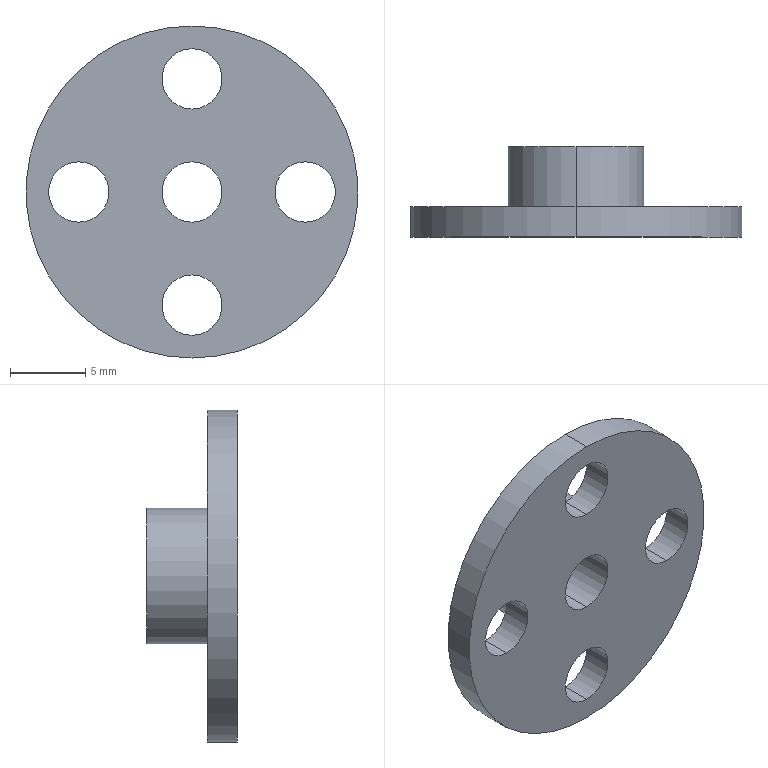Part | SolidWorks | features ICE 2, Extrusion 1 | 1 solid | 17 faces | box 22 x 6 x 22 mm | volume 838.805 mm3 | cylinder 14 | plane 3 | commonest cylinder face diameters 4 x10 9 x2 22 x2
STEP:
#1=CARTESIAN_POINT('',(0.,0.,-2.));
#2=VERTEX_POINT('',#1);
#3=CARTESIAN_POINT('',(0.,0.,2.));
#4=VERTEX_POINT('',#3);
#5=CARTESIAN_POINT('',(0.,0.,0.));
#6=DIRECTION('',(0.,1.,0.));
#7=DIRECTION('',(0.,0.,1.));
#8=AXIS2_PLACEMENT_3D('',#5,#6,#7);
#9=CIRCLE('',#8,2.);
#10=EDGE_CURVE('',#2,#4,#9,.T.);
#11=ORIENTED_EDGE('',*,*,#10,.F.);
#12=CARTESIAN_POINT('',(0.,6.,-2.));
#13=VERTEX_POINT('',#12);
#14=CARTESIAN_POINT('',(0.,0.,-2.));
#15=DIRECTION('',(0.,1.,0.));
#16=VECTOR('',#15,1000.);
#17=LINE('',#14,#16);
#18=EDGE_CURVE('',#2,#13,#17,.T.);
#19=ORIENTED_EDGE('',*,*,#18,.T.);
#20=CARTESIAN_POINT('',(0.,6.,2.));
#21=VERTEX_POINT('',#20);
#22=CARTESIAN_POINT('',(0.,6.,0.));
#23=DIRECTION('',(0.,1.,0.));
#24=DIRECTION('',(0.,0.,1.));
#25=AXIS2_PLACEMENT_3D('',#22,#23,#24);
#26=CIRCLE('',#25,2.);
#27=EDGE_CURVE('',#13,#21,#26,.T.);
#28=ORIENTED_EDGE('',*,*,#27,.T.);
#29=CARTESIAN_POINT('',(0.,0.,2.));
#30=DIRECTION('',(0.,1.,0.));
#31=VECTOR('',#30,1000.);
#32=LINE('',#29,#31);
#33=EDGE_CURVE('',#4,#21,#32,.T.);
#34=ORIENTED_EDGE('',*,*,#33,.F.);
#35=EDGE_LOOP('',(#11,#19,#28,#34));
#36=FACE_OUTER_BOUND('',#35,.T.);
#37=CARTESIAN_POINT('',(0.,0.,0.));
#38=DIRECTION('',(0.,1.,0.));
#39=DIRECTION('',(0.,0.,1.));
#40=AXIS2_PLACEMENT_3D('',#37,#38,#39);
#41=CYLINDRICAL_SURFACE('',#40,2.);
#42=ADVANCED_FACE('',(#36),#41,.F.);
#43=CARTESIAN_POINT('',(0.,6.,4.5));
#44=VERTEX_POINT('',#43);
#45=CARTESIAN_POINT('',(0.,6.,-4.5));
#46=VERTEX_POINT('',#45);
#47=CARTESIAN_POINT('',(0.,6.,0.));
#48=DIRECTION('',(0.,1.,0.));
#49=DIRECTION('',(0.,0.,1.));
#50=AXIS2_PLACEMENT_3D('',#47,#48,#49);
#51=CIRCLE('',#50,4.5);
#52=EDGE_CURVE('',#44,#46,#51,.T.);
#53=ORIENTED_EDGE('',*,*,#52,.F.);
#54=CARTESIAN_POINT('',(0.,2.,4.5));
#55=VERTEX_POINT('',#54);
#56=CARTESIAN_POINT('',(0.,6.,4.5));
#57=DIRECTION('',(0.,-1.,0.));
#58=VECTOR('',#57,1000.);
#59=LINE('',#56,#58);
#60=EDGE_CURVE('',#44,#55,#59,.T.);
#61=ORIENTED_EDGE('',*,*,#60,.T.);
#62=CARTESIAN_POINT('',(0.,2.,-4.5));
#63=VERTEX_POINT('',#62);
#64=CARTESIAN_POINT('',(0.,2.,0.));
#65=DIRECTION('',(0.,1.,0.));
#66=DIRECTION('',(0.,0.,1.));
#67=AXIS2_PLACEMENT_3D('',#64,#65,#66);
#68=CIRCLE('',#67,4.5);
#69=EDGE_CURVE('',#55,#63,#68,.T.);
#70=ORIENTED_EDGE('',*,*,#69,.T.);
#71=CARTESIAN_POINT('',(0.,6.,-4.5));
#72=DIRECTION('',(0.,-1.,0.));
#73=VECTOR('',#72,1000.);
#74=LINE('',#71,#73);
#75=EDGE_CURVE('',#46,#63,#74,.T.);
#76=ORIENTED_EDGE('',*,*,#75,.F.);
#77=EDGE_LOOP('',(#53,#61,#70,#76));
#78=FACE_OUTER_BOUND('',#77,.T.);
#79=CARTESIAN_POINT('',(0.,6.,0.));
#80=DIRECTION('',(0.,-1.,0.));
#81=DIRECTION('',(0.,0.,-1.));
#82=AXIS2_PLACEMENT_3D('',#79,#80,#81);
#83=CYLINDRICAL_SURFACE('',#82,4.5);
#84=ADVANCED_FACE('',(#78),#83,.T.);
#85=CARTESIAN_POINT('',(-7.5,2.,-2.));
#86=VERTEX_POINT('',#85);
#87=CARTESIAN_POINT('',(-7.5,2.,2.));
#88=VERTEX_POINT('',#87);
#89=CARTESIAN_POINT('',(-7.5,2.,0.));
#90=DIRECTION('',(0.,1.,0.));
#91=DIRECTION('',(0.,0.,1.));
#92=AXIS2_PLACEMENT_3D('',#89,#90,#91);
#93=CIRCLE('',#92,2.);
#94=EDGE_CURVE('',#86,#88,#93,.T.);
#95=ORIENTED_EDGE('',*,*,#94,.T.);
#96=CARTESIAN_POINT('',(-7.5,0.,2.));
#97=VERTEX_POINT('',#96);
#98=CARTESIAN_POINT('',(-7.5,2.,2.));
#99=DIRECTION('',(0.,-1.,0.));
#100=VECTOR('',#99,1000.);
#101=LINE('',#98,#100);
#102=EDGE_CURVE('',#88,#97,#101,.T.);
#103=ORIENTED_EDGE('',*,*,#102,.T.);
#104=CARTESIAN_POINT('',(-7.5,0.,-2.));
#105=VERTEX_POINT('',#104);
#106=CARTESIAN_POINT('',(-7.5,0.,0.));
#107=DIRECTION('',(0.,1.,0.));
#108=DIRECTION('',(0.,0.,1.));
#109=AXIS2_PLACEMENT_3D('',#106,#107,#108);
#110=CIRCLE('',#109,2.);
#111=EDGE_CURVE('',#105,#97,#110,.T.);
#112=ORIENTED_EDGE('',*,*,#111,.F.);
#113=CARTESIAN_POINT('',(-7.5,2.,-2.));
#114=DIRECTION('',(0.,-1.,0.));
#115=VECTOR('',#114,1000.);
#116=LINE('',#113,#115);
#117=EDGE_CURVE('',#86,#105,#116,.T.);
#118=ORIENTED_EDGE('',*,*,#117,.F.);
#119=EDGE_LOOP('',(#95,#103,#112,#118));
#120=FACE_OUTER_BOUND('',#119,.T.);
#121=CARTESIAN_POINT('',(-7.5,2.,0.));
#122=DIRECTION('',(0.,-1.,0.));
#123=DIRECTION('',(0.,0.,-1.));
#124=AXIS2_PLACEMENT_3D('',#121,#122,#123);
#125=CYLINDRICAL_SURFACE('',#124,2.);
#126=ADVANCED_FACE('',(#120),#125,.F.);
#127=CARTESIAN_POINT('',(0.,2.,5.5));
#128=VERTEX_POINT('',#127);
#129=CARTESIAN_POINT('',(0.,2.,9.5));
#130=VERTEX_POINT('',#129);
#131=CARTESIAN_POINT('',(0.,2.,7.5));
#132=DIRECTION('',(0.,1.,0.));
#133=DIRECTION('',(0.,0.,1.));
#134=AXIS2_PLACEMENT_3D('',#131,#132,#133);
#135=CIRCLE('',#134,2.);
#136=EDGE_CURVE('',#128,#130,#135,.T.);
#137=ORIENTED_EDGE('',*,*,#136,.T.);
#138=CARTESIAN_POINT('',(0.,0.,9.5));
#139=VERTEX_POINT('',#138);
#140=CARTESIAN_POINT('',(0.,2.,9.5));
#141=DIRECTION('',(0.,-1.,0.));
#142=VECTOR('',#141,1000.);
#143=LINE('',#140,#142);
#144=EDGE_CURVE('',#130,#139,#143,.T.);
#145=ORIENTED_EDGE('',*,*,#144,.T.);
#146=CARTESIAN_POINT('',(0.,0.,5.5));
#147=VERTEX_POINT('',#146);
#148=CARTESIAN_POINT('',(0.,0.,7.5));
#149=DIRECTION('',(0.,1.,0.));
#150=DIRECTION('',(0.,0.,1.));
#151=AXIS2_PLACEMENT_3D('',#148,#149,#150);
#152=CIRCLE('',#151,2.);
#153=EDGE_CURVE('',#147,#139,#152,.T.);
#154=ORIENTED_EDGE('',*,*,#153,.F.);
#155=CARTESIAN_POINT('',(0.,2.,5.5));
#156=DIRECTION('',(0.,-1.,0.));
#157=VECTOR('',#156,1000.);
#158=LINE('',#155,#157);
#159=EDGE_CURVE('',#128,#147,#158,.T.);
#160=ORIENTED_EDGE('',*,*,#159,.F.);
#161=EDGE_LOOP('',(#137,#145,#154,#160));
#162=FACE_OUTER_BOUND('',#161,.T.);
#163=CARTESIAN_POINT('',(0.,2.,7.5));
#164=DIRECTION('',(0.,-1.,0.));
#165=DIRECTION('',(0.,0.,-1.));
#166=AXIS2_PLACEMENT_3D('',#163,#164,#165);
#167=CYLINDRICAL_SURFACE('',#166,2.);
#168=ADVANCED_FACE('',(#162),#167,.F.);
#169=CARTESIAN_POINT('',(7.5,2.,-2.));
#170=VERTEX_POINT('',#169);
#171=CARTESIAN_POINT('',(7.5,2.,2.));
#172=VERTEX_POINT('',#171);
#173=CARTESIAN_POINT('',(7.5,2.,0.));
#174=DIRECTION('',(0.,1.,0.));
#175=DIRECTION('',(0.,0.,1.));
#176=AXIS2_PLACEMENT_3D('',#173,#174,#175);
#177=CIRCLE('',#176,2.);
#178=EDGE_CURVE('',#170,#172,#177,.T.);
#179=ORIENTED_EDGE('',*,*,#178,.T.);
#180=CARTESIAN_POINT('',(7.5,0.,2.));
#181=VERTEX_POINT('',#180);
#182=CARTESIAN_POINT('',(7.5,2.,2.));
#183=DIRECTION('',(0.,-1.,0.));
#184=VECTOR('',#183,1000.);
#185=LINE('',#182,#184);
#186=EDGE_CURVE('',#172,#181,#185,.T.);
#187=ORIENTED_EDGE('',*,*,#186,.T.);
#188=CARTESIAN_POINT('',(7.5,0.,-2.));
#189=VERTEX_POINT('',#188);
#190=CARTESIAN_POINT('',(7.5,0.,0.));
#191=DIRECTION('',(0.,1.,0.));
#192=DIRECTION('',(0.,0.,1.));
#193=AXIS2_PLACEMENT_3D('',#190,#191,#192);
#194=CIRCLE('',#193,2.);
#195=EDGE_CURVE('',#189,#181,#194,.T.);
#196=ORIENTED_EDGE('',*,*,#195,.F.);
#197=CARTESIAN_POINT('',(7.5,2.,-2.));
#198=DIRECTION('',(0.,-1.,0.));
#199=VECTOR('',#198,1000.);
#200=LINE('',#197,#199);
#201=EDGE_CURVE('',#170,#189,#200,.T.);
#202=ORIENTED_EDGE('',*,*,#201,.F.);
#203=EDGE_LOOP('',(#179,#187,#196,#202));
#204=FACE_OUTER_BOUND('',#203,.T.);
#205=CARTESIAN_POINT('',(7.5,2.,0.));
#206=DIRECTION('',(0.,-1.,0.));
#207=DIRECTION('',(0.,0.,-1.));
#208=AXIS2_PLACEMENT_3D('',#205,#206,#207);
#209=CYLINDRICAL_SURFACE('',#208,2.);
#210=ADVANCED_FACE('',(#204),#209,.F.);
#211=CARTESIAN_POINT('',(0.,2.,-9.5));
#212=VERTEX_POINT('',#211);
#213=CARTESIAN_POINT('',(0.,2.,-5.5));
#214=VERTEX_POINT('',#213);
#215=CARTESIAN_POINT('',(0.,2.,-7.5));
#216=DIRECTION('',(0.,1.,0.));
#217=DIRECTION('',(0.,0.,1.));
#218=AXIS2_PLACEMENT_3D('',#215,#216,#217);
#219=CIRCLE('',#218,2.);
#220=EDGE_CURVE('',#212,#214,#219,.T.);
#221=ORIENTED_EDGE('',*,*,#220,.T.);
#222=CARTESIAN_POINT('',(0.,0.,-5.5));
#223=VERTEX_POINT('',#222);
#224=CARTESIAN_POINT('',(0.,2.,-5.5));
#225=DIRECTION('',(0.,-1.,0.));
#226=VECTOR('',#225,1000.);
#227=LINE('',#224,#226);
#228=EDGE_CURVE('',#214,#223,#227,.T.);
#229=ORIENTED_EDGE('',*,*,#228,.T.);
#230=CARTESIAN_POINT('',(0.,0.,-9.5));
#231=VERTEX_POINT('',#230);
#232=CARTESIAN_POINT('',(0.,0.,-7.5));
#233=DIRECTION('',(0.,1.,0.));
#234=DIRECTION('',(0.,0.,1.));
#235=AXIS2_PLACEMENT_3D('',#232,#233,#234);
#236=CIRCLE('',#235,2.);
#237=EDGE_CURVE('',#231,#223,#236,.T.);
#238=ORIENTED_EDGE('',*,*,#237,.F.);
#239=CARTESIAN_POINT('',(0.,2.,-9.5));
#240=DIRECTION('',(0.,-1.,0.));
#241=VECTOR('',#240,1000.);
#242=LINE('',#239,#241);
#243=EDGE_CURVE('',#212,#231,#242,.T.);
#244=ORIENTED_EDGE('',*,*,#243,.F.);
#245=EDGE_LOOP('',(#221,#229,#238,#244));
#246=FACE_OUTER_BOUND('',#245,.T.);
#247=CARTESIAN_POINT('',(0.,2.,-7.5));
#248=DIRECTION('',(0.,-1.,0.));
#249=DIRECTION('',(0.,0.,-1.));
#250=AXIS2_PLACEMENT_3D('',#247,#248,#249);
#251=CYLINDRICAL_SURFACE('',#250,2.);
#252=ADVANCED_FACE('',(#246),#251,.F.);
#253=CARTESIAN_POINT('',(0.,2.,11.));
#254=VERTEX_POINT('',#253);
#255=CARTESIAN_POINT('',(0.,2.,-11.));
#256=VERTEX_POINT('',#255);
#257=CARTESIAN_POINT('',(0.,2.,0.));
#258=DIRECTION('',(0.,1.,0.));
#259=DIRECTION('',(0.,0.,1.));
#260=AXIS2_PLACEMENT_3D('',#257,#258,#259);
#261=CIRCLE('',#260,11.);
#262=EDGE_CURVE('',#254,#256,#261,.T.);
#263=ORIENTED_EDGE('',*,*,#262,.F.);
#264=CARTESIAN_POINT('',(0.,0.,11.));
#265=VERTEX_POINT('',#264);
#266=CARTESIAN_POINT('',(0.,2.,11.));
#267=DIRECTION('',(0.,-1.,0.));
#268=VECTOR('',#267,1000.);
#269=LINE('',#266,#268);
#270=EDGE_CURVE('',#254,#265,#269,.T.);
#271=ORIENTED_EDGE('',*,*,#270,.T.);
#272=CARTESIAN_POINT('',(0.,0.,-11.));
#273=VERTEX_POINT('',#272);
#274=CARTESIAN_POINT('',(0.,0.,0.));
#275=DIRECTION('',(0.,1.,0.));
#276=DIRECTION('',(0.,0.,1.));
#277=AXIS2_PLACEMENT_3D('',#274,#275,#276);
#278=CIRCLE('',#277,11.);
#279=EDGE_CURVE('',#265,#273,#278,.T.);
#280=ORIENTED_EDGE('',*,*,#279,.T.);
#281=CARTESIAN_POINT('',(0.,2.,-11.));
#282=DIRECTION('',(0.,-1.,0.));
#283=VECTOR('',#282,1000.);
#284=LINE('',#281,#283);
#285=EDGE_CURVE('',#256,#273,#284,.T.);
#286=ORIENTED_EDGE('',*,*,#285,.F.);
#287=EDGE_LOOP('',(#263,#271,#280,#286));
#288=FACE_OUTER_BOUND('',#287,.T.);
#289=CARTESIAN_POINT('',(0.,2.,0.));
#290=DIRECTION('',(0.,-1.,0.));
#291=DIRECTION('',(0.,0.,-1.));
#292=AXIS2_PLACEMENT_3D('',#289,#290,#291);
#293=CYLINDRICAL_SURFACE('',#292,11.);
#294=ADVANCED_FACE('',(#288),#293,.T.);
#295=CARTESIAN_POINT('',(0.,2.,0.));
#296=DIRECTION('',(0.,1.,0.));
#297=DIRECTION('',(0.,0.,1.));
#298=AXIS2_PLACEMENT_3D('',#295,#296,#297);
#299=CIRCLE('',#298,4.5);
#300=EDGE_CURVE('',#63,#55,#299,.T.);
#301=ORIENTED_EDGE('',*,*,#300,.F.);
#302=ORIENTED_EDGE('',*,*,#69,.F.);
#303=EDGE_LOOP('',(#301,#302));
#304=FACE_BOUND('',#303,.T.);
#305=ORIENTED_EDGE('',*,*,#136,.F.);
#306=CARTESIAN_POINT('',(0.,2.,7.5));
#307=DIRECTION('',(0.,1.,0.));
#308=DIRECTION('',(0.,0.,1.));
#309=AXIS2_PLACEMENT_3D('',#306,#307,#308);
#310=CIRCLE('',#309,2.);
#311=EDGE_CURVE('',#130,#128,#310,.T.);
#312=ORIENTED_EDGE('',*,*,#311,.F.);
#313=EDGE_LOOP('',(#305,#312));
#314=FACE_BOUND('',#313,.T.);
#315=ORIENTED_EDGE('',*,*,#220,.F.);
#316=CARTESIAN_POINT('',(0.,2.,-7.5));
#317=DIRECTION('',(0.,1.,0.));
#318=DIRECTION('',(0.,0.,1.));
#319=AXIS2_PLACEMENT_3D('',#316,#317,#318);
#320=CIRCLE('',#319,2.);
#321=EDGE_CURVE('',#214,#212,#320,.T.);
#322=ORIENTED_EDGE('',*,*,#321,.F.);
#323=EDGE_LOOP('',(#315,#322));
#324=FACE_BOUND('',#323,.T.);
#325=CARTESIAN_POINT('',(0.,2.,0.));
#326=DIRECTION('',(0.,1.,0.));
#327=DIRECTION('',(0.,0.,1.));
#328=AXIS2_PLACEMENT_3D('',#325,#326,#327);
#329=CIRCLE('',#328,11.);
#330=EDGE_CURVE('',#256,#254,#329,.T.);
#331=ORIENTED_EDGE('',*,*,#330,.T.);
#332=ORIENTED_EDGE('',*,*,#262,.T.);
#333=EDGE_LOOP('',(#331,#332));
#334=FACE_OUTER_BOUND('',#333,.T.);
#335=ORIENTED_EDGE('',*,*,#178,.F.);
#336=CARTESIAN_POINT('',(7.5,2.,0.));
#337=DIRECTION('',(0.,1.,0.));
#338=DIRECTION('',(0.,0.,1.));
#339=AXIS2_PLACEMENT_3D('',#336,#337,#338);
#340=CIRCLE('',#339,2.);
#341=EDGE_CURVE('',#172,#170,#340,.T.);
#342=ORIENTED_EDGE('',*,*,#341,.F.);
#343=EDGE_LOOP('',(#335,#342));
#344=FACE_BOUND('',#343,.T.);
#345=ORIENTED_EDGE('',*,*,#94,.F.);
#346=CARTESIAN_POINT('',(-7.5,2.,0.));
#347=DIRECTION('',(0.,1.,0.));
#348=DIRECTION('',(0.,0.,1.));
#349=AXIS2_PLACEMENT_3D('',#346,#347,#348);
#350=CIRCLE('',#349,2.);
#351=EDGE_CURVE('',#88,#86,#350,.T.);
#352=ORIENTED_EDGE('',*,*,#351,.F.);
#353=EDGE_LOOP('',(#345,#352));
#354=FACE_BOUND('',#353,.T.);
#355=CARTESIAN_POINT('',(0.,2.,0.));
#356=DIRECTION('',(0.,1.,0.));
#357=DIRECTION('',(0.,0.,1.));
#358=AXIS2_PLACEMENT_3D('',#355,#356,#357);
#359=PLANE('',#358);
#360=ADVANCED_FACE('',(#304,#314,#324,#334,#344,#354),#359,.T.);
#361=CARTESIAN_POINT('',(0.,0.,0.));
#362=DIRECTION('',(0.,1.,0.));
#363=DIRECTION('',(0.,0.,1.));
#364=AXIS2_PLACEMENT_3D('',#361,#362,#363);
#365=CIRCLE('',#364,2.);
#366=EDGE_CURVE('',#4,#2,#365,.T.);
#367=ORIENTED_EDGE('',*,*,#366,.T.);
#368=ORIENTED_EDGE('',*,*,#10,.T.);
#369=EDGE_LOOP('',(#367,#368));
#370=FACE_BOUND('',#369,.T.);
#371=CARTESIAN_POINT('',(0.,0.,0.));
#372=DIRECTION('',(0.,1.,0.));
#373=DIRECTION('',(0.,0.,1.));
#374=AXIS2_PLACEMENT_3D('',#371,#372,#373);
#375=CIRCLE('',#374,11.);
#376=EDGE_CURVE('',#273,#265,#375,.T.);
#377=ORIENTED_EDGE('',*,*,#376,.F.);
#378=ORIENTED_EDGE('',*,*,#279,.F.);
#379=EDGE_LOOP('',(#377,#378));
#380=FACE_OUTER_BOUND('',#379,.T.);
#381=ORIENTED_EDGE('',*,*,#237,.T.);
#382=CARTESIAN_POINT('',(0.,0.,-7.5));
#383=DIRECTION('',(0.,1.,0.));
#384=DIRECTION('',(0.,0.,1.));
#385=AXIS2_PLACEMENT_3D('',#382,#383,#384);
#386=CIRCLE('',#385,2.);
#387=EDGE_CURVE('',#223,#231,#386,.T.);
#388=ORIENTED_EDGE('',*,*,#387,.T.);
#389=EDGE_LOOP('',(#381,#388));
#390=FACE_BOUND('',#389,.T.);
#391=ORIENTED_EDGE('',*,*,#195,.T.);
#392=CARTESIAN_POINT('',(7.5,0.,0.));
#393=DIRECTION('',(0.,1.,0.));
#394=DIRECTION('',(0.,0.,1.));
#395=AXIS2_PLACEMENT_3D('',#392,#393,#394);
#396=CIRCLE('',#395,2.);
#397=EDGE_CURVE('',#181,#189,#396,.T.);
#398=ORIENTED_EDGE('',*,*,#397,.T.);
#399=EDGE_LOOP('',(#391,#398));
#400=FACE_BOUND('',#399,.T.);
#401=ORIENTED_EDGE('',*,*,#153,.T.);
#402=CARTESIAN_POINT('',(0.,0.,7.5));
#403=DIRECTION('',(0.,1.,0.));
#404=DIRECTION('',(0.,0.,1.));
#405=AXIS2_PLACEMENT_3D('',#402,#403,#404);
#406=CIRCLE('',#405,2.);
#407=EDGE_CURVE('',#139,#147,#406,.T.);
#408=ORIENTED_EDGE('',*,*,#407,.T.);
#409=EDGE_LOOP('',(#401,#408));
#410=FACE_BOUND('',#409,.T.);
#411=ORIENTED_EDGE('',*,*,#111,.T.);
#412=CARTESIAN_POINT('',(-7.5,0.,0.));
#413=DIRECTION('',(0.,1.,0.));
#414=DIRECTION('',(0.,0.,1.));
#415=AXIS2_PLACEMENT_3D('',#412,#413,#414);
#416=CIRCLE('',#415,2.);
#417=EDGE_CURVE('',#97,#105,#416,.T.);
#418=ORIENTED_EDGE('',*,*,#417,.T.);
#419=EDGE_LOOP('',(#411,#418));
#420=FACE_BOUND('',#419,.T.);
#421=CARTESIAN_POINT('',(0.,0.,0.));
#422=DIRECTION('',(0.,1.,0.));
#423=DIRECTION('',(0.,0.,1.));
#424=AXIS2_PLACEMENT_3D('',#421,#422,#423);
#425=PLANE('',#424);
#426=ADVANCED_FACE('',(#370,#380,#390,#400,#410,#420),#425,.F.);
#427=ORIENTED_EDGE('',*,*,#270,.F.);
#428=ORIENTED_EDGE('',*,*,#330,.F.);
#429=ORIENTED_EDGE('',*,*,#285,.T.);
#430=ORIENTED_EDGE('',*,*,#376,.T.);
#431=EDGE_LOOP('',(#427,#428,#429,#430));
#432=FACE_OUTER_BOUND('',#431,.T.);
#433=CARTESIAN_POINT('',(0.,2.,0.));
#434=DIRECTION('',(0.,-1.,0.));
#435=DIRECTION('',(0.,0.,-1.));
#436=AXIS2_PLACEMENT_3D('',#433,#434,#435);
#437=CYLINDRICAL_SURFACE('',#436,11.);
#438=ADVANCED_FACE('',(#432),#437,.T.);
#439=ORIENTED_EDGE('',*,*,#228,.F.);
#440=ORIENTED_EDGE('',*,*,#321,.T.);
#441=ORIENTED_EDGE('',*,*,#243,.T.);
#442=ORIENTED_EDGE('',*,*,#387,.F.);
#443=EDGE_LOOP('',(#439,#440,#441,#442));
#444=FACE_OUTER_BOUND('',#443,.T.);
#445=CARTESIAN_POINT('',(0.,2.,-7.5));
#446=DIRECTION('',(0.,-1.,0.));
#447=DIRECTION('',(0.,0.,-1.));
#448=AXIS2_PLACEMENT_3D('',#445,#446,#447);
#449=CYLINDRICAL_SURFACE('',#448,2.);
#450=ADVANCED_FACE('',(#444),#449,.F.);
#451=ORIENTED_EDGE('',*,*,#186,.F.);
#452=ORIENTED_EDGE('',*,*,#341,.T.);
#453=ORIENTED_EDGE('',*,*,#201,.T.);
#454=ORIENTED_EDGE('',*,*,#397,.F.);
#455=EDGE_LOOP('',(#451,#452,#453,#454));
#456=FACE_OUTER_BOUND('',#455,.T.);
#457=CARTESIAN_POINT('',(7.5,2.,0.));
#458=DIRECTION('',(0.,-1.,0.));
#459=DIRECTION('',(0.,0.,-1.));
#460=AXIS2_PLACEMENT_3D('',#457,#458,#459);
#461=CYLINDRICAL_SURFACE('',#460,2.);
#462=ADVANCED_FACE('',(#456),#461,.F.);
#463=ORIENTED_EDGE('',*,*,#144,.F.);
#464=ORIENTED_EDGE('',*,*,#311,.T.);
#465=ORIENTED_EDGE('',*,*,#159,.T.);
#466=ORIENTED_EDGE('',*,*,#407,.F.);
#467=EDGE_LOOP('',(#463,#464,#465,#466));
#468=FACE_OUTER_BOUND('',#467,.T.);
#469=CARTESIAN_POINT('',(0.,2.,7.5));
#470=DIRECTION('',(0.,-1.,0.));
#471=DIRECTION('',(0.,0.,-1.));
#472=AXIS2_PLACEMENT_3D('',#469,#470,#471);
#473=CYLINDRICAL_SURFACE('',#472,2.);
#474=ADVANCED_FACE('',(#468),#473,.F.);
#475=ORIENTED_EDGE('',*,*,#102,.F.);
#476=ORIENTED_EDGE('',*,*,#351,.T.);
#477=ORIENTED_EDGE('',*,*,#117,.T.);
#478=ORIENTED_EDGE('',*,*,#417,.F.);
#479=EDGE_LOOP('',(#475,#476,#477,#478));
#480=FACE_OUTER_BOUND('',#479,.T.);
#481=CARTESIAN_POINT('',(-7.5,2.,0.));
#482=DIRECTION('',(0.,-1.,0.));
#483=DIRECTION('',(0.,0.,-1.));
#484=AXIS2_PLACEMENT_3D('',#481,#482,#483);
#485=CYLINDRICAL_SURFACE('',#484,2.);
#486=ADVANCED_FACE('',(#480),#485,.F.);
#487=ORIENTED_EDGE('',*,*,#60,.F.);
#488=CARTESIAN_POINT('',(0.,6.,0.));
#489=DIRECTION('',(0.,1.,0.));
#490=DIRECTION('',(0.,0.,1.));
#491=AXIS2_PLACEMENT_3D('',#488,#489,#490);
#492=CIRCLE('',#491,4.5);
#493=EDGE_CURVE('',#46,#44,#492,.T.);
#494=ORIENTED_EDGE('',*,*,#493,.F.);
#495=ORIENTED_EDGE('',*,*,#75,.T.);
#496=ORIENTED_EDGE('',*,*,#300,.T.);
#497=EDGE_LOOP('',(#487,#494,#495,#496));
#498=FACE_OUTER_BOUND('',#497,.T.);
#499=CARTESIAN_POINT('',(0.,6.,0.));
#500=DIRECTION('',(0.,-1.,0.));
#501=DIRECTION('',(0.,0.,-1.));
#502=AXIS2_PLACEMENT_3D('',#499,#500,#501);
#503=CYLINDRICAL_SURFACE('',#502,4.5);
#504=ADVANCED_FACE('',(#498),#503,.T.);
#505=CARTESIAN_POINT('',(0.,6.,0.));
#506=DIRECTION('',(0.,1.,0.));
#507=DIRECTION('',(0.,0.,1.));
#508=AXIS2_PLACEMENT_3D('',#505,#506,#507);
#509=CIRCLE('',#508,2.);
#510=EDGE_CURVE('',#21,#13,#509,.T.);
#511=ORIENTED_EDGE('',*,*,#510,.F.);
#512=ORIENTED_EDGE('',*,*,#27,.F.);
#513=EDGE_LOOP('',(#511,#512));
#514=FACE_BOUND('',#513,.T.);
#515=ORIENTED_EDGE('',*,*,#493,.T.);
#516=ORIENTED_EDGE('',*,*,#52,.T.);
#517=EDGE_LOOP('',(#515,#516));
#518=FACE_OUTER_BOUND('',#517,.T.);
#519=CARTESIAN_POINT('',(0.,6.,0.));
#520=DIRECTION('',(0.,1.,0.));
#521=DIRECTION('',(0.,0.,1.));
#522=AXIS2_PLACEMENT_3D('',#519,#520,#521);
#523=PLANE('',#522);
#524=ADVANCED_FACE('',(#514,#518),#523,.T.);
#525=ORIENTED_EDGE('',*,*,#18,.F.);
#526=ORIENTED_EDGE('',*,*,#366,.F.);
#527=ORIENTED_EDGE('',*,*,#33,.T.);
#528=ORIENTED_EDGE('',*,*,#510,.T.);
#529=EDGE_LOOP('',(#525,#526,#527,#528));
#530=FACE_OUTER_BOUND('',#529,.T.);
#531=CARTESIAN_POINT('',(0.,0.,0.));
#532=DIRECTION('',(0.,1.,0.));
#533=DIRECTION('',(0.,0.,1.));
#534=AXIS2_PLACEMENT_3D('',#531,#532,#533);
#535=CYLINDRICAL_SURFACE('',#534,2.);
#536=ADVANCED_FACE('',(#530),#535,.F.);
#537=CLOSED_SHELL('',(#42,#84,#126,#168,#210,#252,#294,#360,#426,#438,#450,#462,#474,#486,#504,#524,#536));
#538=MANIFOLD_SOLID_BREP('',#537);
#539=CARTESIAN_POINT('',(0.,0.,0.));
#540=DIRECTION('',(0.,0.,1.));
#541=DIRECTION('',(1.,0.,0.));
#542=AXIS2_PLACEMENT_3D('',#539,#540,#541);
#543=(LENGTH_UNIT()NAMED_UNIT(*)SI_UNIT(.MILLI.,.METRE.));
#544=UNCERTAINTY_MEASURE_WITH_UNIT(LENGTH_MEASURE(0.00001),#543,'','');
#545=(NAMED_UNIT(*)PLANE_ANGLE_UNIT()SI_UNIT($,.RADIAN.));
#546=(NAMED_UNIT(*)SI_UNIT($,.STERADIAN.)SOLID_ANGLE_UNIT());
#547=(GEOMETRIC_REPRESENTATION_CONTEXT(3)GLOBAL_UNCERTAINTY_ASSIGNED_CONTEXT((#544))GLOBAL_UNIT_ASSIGNED_CONTEXT((#543,#545,#546))REPRESENTATION_CONTEXT('',''));
#548=ADVANCED_BREP_SHAPE_REPRESENTATION('',(#538,#542),#547);